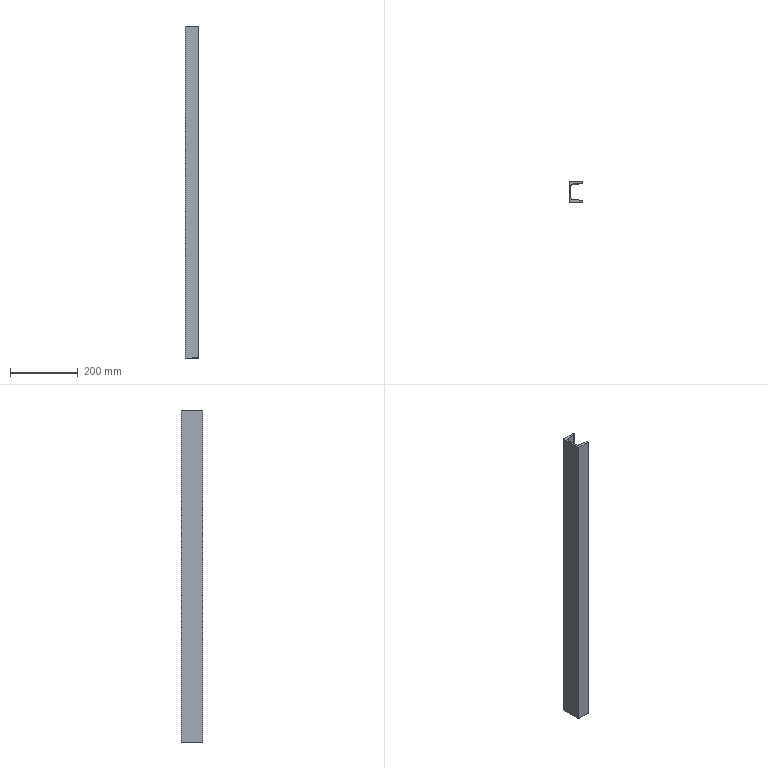Part | STEP file | 750038231 | 1 solid | 14 faces | box 40 x 63 x 982 mm | volume 829365 mm3 | plane 10 | cylinder 4 | commonest cylinder face diameters 7.6 x2 15 x2
STEP:
#1=CARTESIAN_POINT('',(0.,0.,491.));
#2=VERTEX_POINT('',#1);
#3=CARTESIAN_POINT('',(0.,0.,-491.));
#4=VERTEX_POINT('',#3);
#5=CARTESIAN_POINT('',(0.,0.,491.));
#6=DIRECTION('',(0.,0.,-1.));
#7=VECTOR('',#6,1000.);
#8=LINE('',#5,#7);
#9=EDGE_CURVE('',#2,#4,#8,.T.);
#10=ORIENTED_EDGE('',*,*,#9,.F.);
#11=CARTESIAN_POINT('',(0.,63.,491.));
#12=VERTEX_POINT('',#11);
#13=CARTESIAN_POINT('',(0.,63.,491.));
#14=DIRECTION('',(0.,-1.,0.));
#15=VECTOR('',#14,1000.);
#16=LINE('',#13,#15);
#17=EDGE_CURVE('',#12,#2,#16,.T.);
#18=ORIENTED_EDGE('',*,*,#17,.F.);
#19=CARTESIAN_POINT('',(0.,63.,-491.));
#20=VERTEX_POINT('',#19);
#21=CARTESIAN_POINT('',(0.,63.,491.));
#22=DIRECTION('',(0.,0.,1.));
#23=VECTOR('',#22,1000.);
#24=LINE('',#21,#23);
#25=EDGE_CURVE('',#20,#12,#24,.T.);
#26=ORIENTED_EDGE('',*,*,#25,.F.);
#27=CARTESIAN_POINT('',(0.,63.,-491.));
#28=DIRECTION('',(0.,1.,0.));
#29=VECTOR('',#28,1000.);
#30=LINE('',#27,#29);
#31=EDGE_CURVE('',#4,#20,#30,.T.);
#32=ORIENTED_EDGE('',*,*,#31,.F.);
#33=EDGE_LOOP('',(#10,#18,#26,#32));
#34=FACE_OUTER_BOUND('',#33,.T.);
#35=CARTESIAN_POINT('',(0.,63.,491.));
#36=DIRECTION('',(1.,0.,0.));
#37=DIRECTION('',(0.,0.,-1.));
#38=AXIS2_PLACEMENT_3D('',#35,#36,#37);
#39=PLANE('',#38);
#40=ADVANCED_FACE('',(#34),#39,.F.);
#41=CARTESIAN_POINT('',(40.,63.,-491.));
#42=VERTEX_POINT('',#41);
#43=CARTESIAN_POINT('',(36.2,63.,-491.));
#44=DIRECTION('',(-1.,0.,0.));
#45=VECTOR('',#44,1000.);
#46=LINE('',#43,#45);
#47=EDGE_CURVE('',#42,#20,#46,.T.);
#48=ORIENTED_EDGE('',*,*,#47,.F.);
#49=CARTESIAN_POINT('',(40.,60.699,-491.));
#50=VERTEX_POINT('',#49);
#51=CARTESIAN_POINT('',(40.,2.301,-491.));
#52=DIRECTION('',(0.,1.,0.));
#53=VECTOR('',#52,1000.);
#54=LINE('',#51,#53);
#55=EDGE_CURVE('',#50,#42,#54,.T.);
#56=ORIENTED_EDGE('',*,*,#55,.F.);
#57=CARTESIAN_POINT('',(36.578,56.918,-491.));
#58=VERTEX_POINT('',#57);
#59=CARTESIAN_POINT('',(36.2,60.699,-491.));
#60=DIRECTION('',(0.,0.,1.));
#61=DIRECTION('',(-1.,0.,0.));
#62=AXIS2_PLACEMENT_3D('',#59,#60,#61);
#63=CIRCLE('',#62,3.8);
#64=EDGE_CURVE('',#58,#50,#63,.T.);
#65=ORIENTED_EDGE('',*,*,#64,.F.);
#66=CARTESIAN_POINT('',(11.554,54.415,-491.));
#67=VERTEX_POINT('',#66);
#68=CARTESIAN_POINT('',(11.554,54.415,-491.));
#69=DIRECTION('',(0.995,0.0995,0.));
#70=VECTOR('',#69,1000.);
#71=LINE('',#68,#70);
#72=EDGE_CURVE('',#67,#58,#71,.T.);
#73=ORIENTED_EDGE('',*,*,#72,.F.);
#74=CARTESIAN_POINT('',(4.8,46.953,-491.));
#75=VERTEX_POINT('',#74);
#76=CARTESIAN_POINT('',(12.3,46.953,-491.));
#77=DIRECTION('',(0.,0.,-1.));
#78=DIRECTION('',(-1.,0.,0.));
#79=AXIS2_PLACEMENT_3D('',#76,#77,#78);
#80=CIRCLE('',#79,7.5);
#81=EDGE_CURVE('',#75,#67,#80,.T.);
#82=ORIENTED_EDGE('',*,*,#81,.F.);
#83=CARTESIAN_POINT('',(4.8,16.047,-491.));
#84=VERTEX_POINT('',#83);
#85=CARTESIAN_POINT('',(4.8,2.301,-491.));
#86=DIRECTION('',(0.,1.,0.));
#87=VECTOR('',#86,1000.);
#88=LINE('',#85,#87);
#89=EDGE_CURVE('',#84,#75,#88,.T.);
#90=ORIENTED_EDGE('',*,*,#89,.F.);
#91=CARTESIAN_POINT('',(11.554,8.585,-491.));
#92=VERTEX_POINT('',#91);
#93=CARTESIAN_POINT('',(12.3,16.047,-491.));
#94=DIRECTION('',(0.,0.,-1.));
#95=DIRECTION('',(-1.,0.,0.));
#96=AXIS2_PLACEMENT_3D('',#93,#94,#95);
#97=CIRCLE('',#96,7.5);
#98=EDGE_CURVE('',#92,#84,#97,.T.);
#99=ORIENTED_EDGE('',*,*,#98,.F.);
#100=CARTESIAN_POINT('',(36.578,6.082,-491.));
#101=VERTEX_POINT('',#100);
#102=CARTESIAN_POINT('',(36.578,6.082,-491.));
#103=DIRECTION('',(-0.995,0.0995,0.));
#104=VECTOR('',#103,1000.);
#105=LINE('',#102,#104);
#106=EDGE_CURVE('',#101,#92,#105,.T.);
#107=ORIENTED_EDGE('',*,*,#106,.F.);
#108=CARTESIAN_POINT('',(40.,2.301,-491.));
#109=VERTEX_POINT('',#108);
#110=CARTESIAN_POINT('',(36.2,2.301,-491.));
#111=DIRECTION('',(0.,0.,1.));
#112=DIRECTION('',(-1.,0.,0.));
#113=AXIS2_PLACEMENT_3D('',#110,#111,#112);
#114=CIRCLE('',#113,3.8);
#115=EDGE_CURVE('',#109,#101,#114,.T.);
#116=ORIENTED_EDGE('',*,*,#115,.F.);
#117=CARTESIAN_POINT('',(40.,0.,-491.));
#118=VERTEX_POINT('',#117);
#119=CARTESIAN_POINT('',(40.,2.301,-491.));
#120=DIRECTION('',(0.,1.,0.));
#121=VECTOR('',#120,1000.);
#122=LINE('',#119,#121);
#123=EDGE_CURVE('',#118,#109,#122,.T.);
#124=ORIENTED_EDGE('',*,*,#123,.F.);
#125=CARTESIAN_POINT('',(36.2,0.,-491.));
#126=DIRECTION('',(1.,0.,0.));
#127=VECTOR('',#126,1000.);
#128=LINE('',#125,#127);
#129=EDGE_CURVE('',#4,#118,#128,.T.);
#130=ORIENTED_EDGE('',*,*,#129,.F.);
#131=ORIENTED_EDGE('',*,*,#31,.T.);
#132=EDGE_LOOP('',(#48,#56,#65,#73,#82,#90,#99,#107,#116,#124,#130,#131));
#133=FACE_OUTER_BOUND('',#132,.T.);
#134=CARTESIAN_POINT('',(36.2,2.301,-491.));
#135=DIRECTION('',(0.,0.,1.));
#136=DIRECTION('',(1.,0.,0.));
#137=AXIS2_PLACEMENT_3D('',#134,#135,#136);
#138=PLANE('',#137);
#139=ADVANCED_FACE('',(#133),#138,.F.);
#140=CARTESIAN_POINT('',(40.,0.,491.));
#141=VERTEX_POINT('',#140);
#142=CARTESIAN_POINT('',(40.,0.,491.));
#143=DIRECTION('',(0.,0.,-1.));
#144=VECTOR('',#143,1000.);
#145=LINE('',#142,#144);
#146=EDGE_CURVE('',#141,#118,#145,.T.);
#147=ORIENTED_EDGE('',*,*,#146,.F.);
#148=CARTESIAN_POINT('',(0.,0.,491.));
#149=DIRECTION('',(1.,0.,0.));
#150=VECTOR('',#149,1000.);
#151=LINE('',#148,#150);
#152=EDGE_CURVE('',#2,#141,#151,.T.);
#153=ORIENTED_EDGE('',*,*,#152,.F.);
#154=ORIENTED_EDGE('',*,*,#9,.T.);
#155=ORIENTED_EDGE('',*,*,#129,.T.);
#156=EDGE_LOOP('',(#147,#153,#154,#155));
#157=FACE_OUTER_BOUND('',#156,.T.);
#158=CARTESIAN_POINT('',(0.,0.,491.));
#159=DIRECTION('',(0.,1.,0.));
#160=DIRECTION('',(0.,0.,1.));
#161=AXIS2_PLACEMENT_3D('',#158,#159,#160);
#162=PLANE('',#161);
#163=ADVANCED_FACE('',(#157),#162,.F.);
#164=CARTESIAN_POINT('',(40.,60.699,491.));
#165=VERTEX_POINT('',#164);
#166=CARTESIAN_POINT('',(40.,63.,491.));
#167=VERTEX_POINT('',#166);
#168=CARTESIAN_POINT('',(40.,2.301,491.));
#169=DIRECTION('',(0.,1.,0.));
#170=VECTOR('',#169,1000.);
#171=LINE('',#168,#170);
#172=EDGE_CURVE('',#165,#167,#171,.T.);
#173=ORIENTED_EDGE('',*,*,#172,.T.);
#174=CARTESIAN_POINT('',(36.2,63.,491.));
#175=DIRECTION('',(-1.,0.,0.));
#176=VECTOR('',#175,1000.);
#177=LINE('',#174,#176);
#178=EDGE_CURVE('',#167,#12,#177,.T.);
#179=ORIENTED_EDGE('',*,*,#178,.T.);
#180=ORIENTED_EDGE('',*,*,#17,.T.);
#181=ORIENTED_EDGE('',*,*,#152,.T.);
#182=CARTESIAN_POINT('',(40.,2.301,491.));
#183=VERTEX_POINT('',#182);
#184=CARTESIAN_POINT('',(40.,2.301,491.));
#185=DIRECTION('',(0.,1.,0.));
#186=VECTOR('',#185,1000.);
#187=LINE('',#184,#186);
#188=EDGE_CURVE('',#141,#183,#187,.T.);
#189=ORIENTED_EDGE('',*,*,#188,.T.);
#190=CARTESIAN_POINT('',(36.578,6.082,491.));
#191=VERTEX_POINT('',#190);
#192=CARTESIAN_POINT('',(36.2,2.301,491.));
#193=DIRECTION('',(0.,0.,1.));
#194=DIRECTION('',(-1.,0.,0.));
#195=AXIS2_PLACEMENT_3D('',#192,#193,#194);
#196=CIRCLE('',#195,3.8);
#197=EDGE_CURVE('',#183,#191,#196,.T.);
#198=ORIENTED_EDGE('',*,*,#197,.T.);
#199=CARTESIAN_POINT('',(11.554,8.585,491.));
#200=VERTEX_POINT('',#199);
#201=CARTESIAN_POINT('',(36.578,6.082,491.));
#202=DIRECTION('',(-0.995,0.0995,0.));
#203=VECTOR('',#202,1000.);
#204=LINE('',#201,#203);
#205=EDGE_CURVE('',#191,#200,#204,.T.);
#206=ORIENTED_EDGE('',*,*,#205,.T.);
#207=CARTESIAN_POINT('',(4.8,16.047,491.));
#208=VERTEX_POINT('',#207);
#209=CARTESIAN_POINT('',(12.3,16.047,491.));
#210=DIRECTION('',(0.,0.,-1.));
#211=DIRECTION('',(-1.,0.,0.));
#212=AXIS2_PLACEMENT_3D('',#209,#210,#211);
#213=CIRCLE('',#212,7.5);
#214=EDGE_CURVE('',#200,#208,#213,.T.);
#215=ORIENTED_EDGE('',*,*,#214,.T.);
#216=CARTESIAN_POINT('',(4.8,46.953,491.));
#217=VERTEX_POINT('',#216);
#218=CARTESIAN_POINT('',(4.8,2.301,491.));
#219=DIRECTION('',(0.,1.,0.));
#220=VECTOR('',#219,1000.);
#221=LINE('',#218,#220);
#222=EDGE_CURVE('',#208,#217,#221,.T.);
#223=ORIENTED_EDGE('',*,*,#222,.T.);
#224=CARTESIAN_POINT('',(11.554,54.415,491.));
#225=VERTEX_POINT('',#224);
#226=CARTESIAN_POINT('',(12.3,46.953,491.));
#227=DIRECTION('',(0.,0.,-1.));
#228=DIRECTION('',(-1.,0.,0.));
#229=AXIS2_PLACEMENT_3D('',#226,#227,#228);
#230=CIRCLE('',#229,7.5);
#231=EDGE_CURVE('',#217,#225,#230,.T.);
#232=ORIENTED_EDGE('',*,*,#231,.T.);
#233=CARTESIAN_POINT('',(36.578,56.918,491.));
#234=VERTEX_POINT('',#233);
#235=CARTESIAN_POINT('',(11.554,54.415,491.));
#236=DIRECTION('',(0.995,0.0995,0.));
#237=VECTOR('',#236,1000.);
#238=LINE('',#235,#237);
#239=EDGE_CURVE('',#225,#234,#238,.T.);
#240=ORIENTED_EDGE('',*,*,#239,.T.);
#241=CARTESIAN_POINT('',(36.2,60.699,491.));
#242=DIRECTION('',(0.,0.,1.));
#243=DIRECTION('',(-1.,0.,0.));
#244=AXIS2_PLACEMENT_3D('',#241,#242,#243);
#245=CIRCLE('',#244,3.8);
#246=EDGE_CURVE('',#234,#165,#245,.T.);
#247=ORIENTED_EDGE('',*,*,#246,.T.);
#248=EDGE_LOOP('',(#173,#179,#180,#181,#189,#198,#206,#215,#223,#232,#240,#247));
#249=FACE_OUTER_BOUND('',#248,.T.);
#250=CARTESIAN_POINT('',(36.2,2.301,491.));
#251=DIRECTION('',(0.,0.,1.));
#252=DIRECTION('',(1.,0.,0.));
#253=AXIS2_PLACEMENT_3D('',#250,#251,#252);
#254=PLANE('',#253);
#255=ADVANCED_FACE('',(#249),#254,.T.);
#256=ORIENTED_EDGE('',*,*,#25,.T.);
#257=ORIENTED_EDGE('',*,*,#178,.F.);
#258=CARTESIAN_POINT('',(40.,63.,491.));
#259=DIRECTION('',(0.,0.,1.));
#260=VECTOR('',#259,1000.);
#261=LINE('',#258,#260);
#262=EDGE_CURVE('',#42,#167,#261,.T.);
#263=ORIENTED_EDGE('',*,*,#262,.F.);
#264=ORIENTED_EDGE('',*,*,#47,.T.);
#265=EDGE_LOOP('',(#256,#257,#263,#264));
#266=FACE_OUTER_BOUND('',#265,.T.);
#267=CARTESIAN_POINT('',(40.,63.,491.));
#268=DIRECTION('',(0.,-1.,0.));
#269=DIRECTION('',(0.,0.,-1.));
#270=AXIS2_PLACEMENT_3D('',#267,#268,#269);
#271=PLANE('',#270);
#272=ADVANCED_FACE('',(#266),#271,.F.);
#273=ORIENTED_EDGE('',*,*,#262,.T.);
#274=ORIENTED_EDGE('',*,*,#172,.F.);
#275=CARTESIAN_POINT('',(40.,60.699,491.));
#276=DIRECTION('',(0.,0.,1.));
#277=VECTOR('',#276,1000.);
#278=LINE('',#275,#277);
#279=EDGE_CURVE('',#50,#165,#278,.T.);
#280=ORIENTED_EDGE('',*,*,#279,.F.);
#281=ORIENTED_EDGE('',*,*,#55,.T.);
#282=EDGE_LOOP('',(#273,#274,#280,#281));
#283=FACE_OUTER_BOUND('',#282,.T.);
#284=CARTESIAN_POINT('',(40.,60.699,491.));
#285=DIRECTION('',(-1.,0.,0.));
#286=DIRECTION('',(0.,-1.,0.));
#287=AXIS2_PLACEMENT_3D('',#284,#285,#286);
#288=PLANE('',#287);
#289=ADVANCED_FACE('',(#283),#288,.F.);
#290=ORIENTED_EDGE('',*,*,#246,.F.);
#291=CARTESIAN_POINT('',(36.578,56.918,491.));
#292=DIRECTION('',(0.,0.,-1.));
#293=VECTOR('',#292,1000.);
#294=LINE('',#291,#293);
#295=EDGE_CURVE('',#234,#58,#294,.T.);
#296=ORIENTED_EDGE('',*,*,#295,.T.);
#297=ORIENTED_EDGE('',*,*,#64,.T.);
#298=ORIENTED_EDGE('',*,*,#279,.T.);
#299=EDGE_LOOP('',(#290,#296,#297,#298));
#300=FACE_OUTER_BOUND('',#299,.T.);
#301=CARTESIAN_POINT('',(36.2,60.699,491.));
#302=DIRECTION('',(0.,0.,-1.));
#303=DIRECTION('',(-1.,0.,0.));
#304=AXIS2_PLACEMENT_3D('',#301,#302,#303);
#305=CYLINDRICAL_SURFACE('',#304,3.8);
#306=ADVANCED_FACE('',(#300),#305,.T.);
#307=ORIENTED_EDGE('',*,*,#295,.F.);
#308=ORIENTED_EDGE('',*,*,#239,.F.);
#309=CARTESIAN_POINT('',(11.554,54.415,491.));
#310=DIRECTION('',(0.,0.,1.));
#311=VECTOR('',#310,1000.);
#312=LINE('',#309,#311);
#313=EDGE_CURVE('',#67,#225,#312,.T.);
#314=ORIENTED_EDGE('',*,*,#313,.F.);
#315=ORIENTED_EDGE('',*,*,#72,.T.);
#316=EDGE_LOOP('',(#307,#308,#314,#315));
#317=FACE_OUTER_BOUND('',#316,.T.);
#318=CARTESIAN_POINT('',(11.554,54.415,491.));
#319=DIRECTION('',(-0.0995,0.995,0.));
#320=DIRECTION('',(-0.995,-0.0995,0.));
#321=AXIS2_PLACEMENT_3D('',#318,#319,#320);
#322=PLANE('',#321);
#323=ADVANCED_FACE('',(#317),#322,.F.);
#324=ORIENTED_EDGE('',*,*,#313,.T.);
#325=ORIENTED_EDGE('',*,*,#231,.F.);
#326=CARTESIAN_POINT('',(4.8,46.953,491.));
#327=DIRECTION('',(0.,0.,1.));
#328=VECTOR('',#327,1000.);
#329=LINE('',#326,#328);
#330=EDGE_CURVE('',#75,#217,#329,.T.);
#331=ORIENTED_EDGE('',*,*,#330,.F.);
#332=ORIENTED_EDGE('',*,*,#81,.T.);
#333=EDGE_LOOP('',(#324,#325,#331,#332));
#334=FACE_OUTER_BOUND('',#333,.T.);
#335=CARTESIAN_POINT('',(12.3,46.953,491.));
#336=DIRECTION('',(0.,0.,-1.));
#337=DIRECTION('',(-1.,0.,0.));
#338=AXIS2_PLACEMENT_3D('',#335,#336,#337);
#339=CYLINDRICAL_SURFACE('',#338,7.5);
#340=ADVANCED_FACE('',(#334),#339,.F.);
#341=ORIENTED_EDGE('',*,*,#330,.T.);
#342=ORIENTED_EDGE('',*,*,#222,.F.);
#343=CARTESIAN_POINT('',(4.8,16.047,491.));
#344=DIRECTION('',(0.,0.,1.));
#345=VECTOR('',#344,1000.);
#346=LINE('',#343,#345);
#347=EDGE_CURVE('',#84,#208,#346,.T.);
#348=ORIENTED_EDGE('',*,*,#347,.F.);
#349=ORIENTED_EDGE('',*,*,#89,.T.);
#350=EDGE_LOOP('',(#341,#342,#348,#349));
#351=FACE_OUTER_BOUND('',#350,.T.);
#352=CARTESIAN_POINT('',(4.8,16.047,491.));
#353=DIRECTION('',(-1.,0.,0.));
#354=DIRECTION('',(0.,-1.,0.));
#355=AXIS2_PLACEMENT_3D('',#352,#353,#354);
#356=PLANE('',#355);
#357=ADVANCED_FACE('',(#351),#356,.F.);
#358=ORIENTED_EDGE('',*,*,#347,.T.);
#359=ORIENTED_EDGE('',*,*,#214,.F.);
#360=CARTESIAN_POINT('',(11.554,8.585,491.));
#361=DIRECTION('',(0.,0.,1.));
#362=VECTOR('',#361,1000.);
#363=LINE('',#360,#362);
#364=EDGE_CURVE('',#92,#200,#363,.T.);
#365=ORIENTED_EDGE('',*,*,#364,.F.);
#366=ORIENTED_EDGE('',*,*,#98,.T.);
#367=EDGE_LOOP('',(#358,#359,#365,#366));
#368=FACE_OUTER_BOUND('',#367,.T.);
#369=CARTESIAN_POINT('',(12.3,16.047,491.));
#370=DIRECTION('',(0.,0.,-1.));
#371=DIRECTION('',(-1.,0.,0.));
#372=AXIS2_PLACEMENT_3D('',#369,#370,#371);
#373=CYLINDRICAL_SURFACE('',#372,7.5);
#374=ADVANCED_FACE('',(#368),#373,.F.);
#375=ORIENTED_EDGE('',*,*,#364,.T.);
#376=ORIENTED_EDGE('',*,*,#205,.F.);
#377=CARTESIAN_POINT('',(36.578,6.082,491.));
#378=DIRECTION('',(0.,0.,1.));
#379=VECTOR('',#378,1000.);
#380=LINE('',#377,#379);
#381=EDGE_CURVE('',#101,#191,#380,.T.);
#382=ORIENTED_EDGE('',*,*,#381,.F.);
#383=ORIENTED_EDGE('',*,*,#106,.T.);
#384=EDGE_LOOP('',(#375,#376,#382,#383));
#385=FACE_OUTER_BOUND('',#384,.T.);
#386=CARTESIAN_POINT('',(36.578,6.082,491.));
#387=DIRECTION('',(-0.0995,-0.995,0.));
#388=DIRECTION('',(0.995,-0.0995,0.));
#389=AXIS2_PLACEMENT_3D('',#386,#387,#388);
#390=PLANE('',#389);
#391=ADVANCED_FACE('',(#385),#390,.F.);
#392=ORIENTED_EDGE('',*,*,#197,.F.);
#393=CARTESIAN_POINT('',(40.,2.301,491.));
#394=DIRECTION('',(0.,0.,-1.));
#395=VECTOR('',#394,1000.);
#396=LINE('',#393,#395);
#397=EDGE_CURVE('',#183,#109,#396,.T.);
#398=ORIENTED_EDGE('',*,*,#397,.T.);
#399=ORIENTED_EDGE('',*,*,#115,.T.);
#400=ORIENTED_EDGE('',*,*,#381,.T.);
#401=EDGE_LOOP('',(#392,#398,#399,#400));
#402=FACE_OUTER_BOUND('',#401,.T.);
#403=CARTESIAN_POINT('',(36.2,2.301,491.));
#404=DIRECTION('',(0.,0.,-1.));
#405=DIRECTION('',(-1.,0.,0.));
#406=AXIS2_PLACEMENT_3D('',#403,#404,#405);
#407=CYLINDRICAL_SURFACE('',#406,3.8);
#408=ADVANCED_FACE('',(#402),#407,.T.);
#409=ORIENTED_EDGE('',*,*,#397,.F.);
#410=ORIENTED_EDGE('',*,*,#188,.F.);
#411=ORIENTED_EDGE('',*,*,#146,.T.);
#412=ORIENTED_EDGE('',*,*,#123,.T.);
#413=EDGE_LOOP('',(#409,#410,#411,#412));
#414=FACE_OUTER_BOUND('',#413,.T.);
#415=CARTESIAN_POINT('',(40.,0.,491.));
#416=DIRECTION('',(-1.,0.,0.));
#417=DIRECTION('',(0.,0.,1.));
#418=AXIS2_PLACEMENT_3D('',#415,#416,#417);
#419=PLANE('',#418);
#420=ADVANCED_FACE('',(#414),#419,.F.);
#421=CLOSED_SHELL('',(#40,#139,#163,#255,#272,#289,#306,#323,#340,#357,#374,#391,#408,#420));
#422=MANIFOLD_SOLID_BREP('',#421);
#423=CARTESIAN_POINT('',(0.,0.,0.));
#424=DIRECTION('',(0.,0.,1.));
#425=DIRECTION('',(1.,0.,0.));
#426=AXIS2_PLACEMENT_3D('',#423,#424,#425);
#427=(LENGTH_UNIT()NAMED_UNIT(*)SI_UNIT(.MILLI.,.METRE.));
#428=UNCERTAINTY_MEASURE_WITH_UNIT(LENGTH_MEASURE(0.00001),#427,'','');
#429=(NAMED_UNIT(*)PLANE_ANGLE_UNIT()SI_UNIT($,.RADIAN.));
#430=(NAMED_UNIT(*)SI_UNIT($,.STERADIAN.)SOLID_ANGLE_UNIT());
#431=(GEOMETRIC_REPRESENTATION_CONTEXT(3)GLOBAL_UNCERTAINTY_ASSIGNED_CONTEXT((#428))GLOBAL_UNIT_ASSIGNED_CONTEXT((#427,#429,#430))REPRESENTATION_CONTEXT('',''));
#432=ADVANCED_BREP_SHAPE_REPRESENTATION('',(#422,#426),#431);